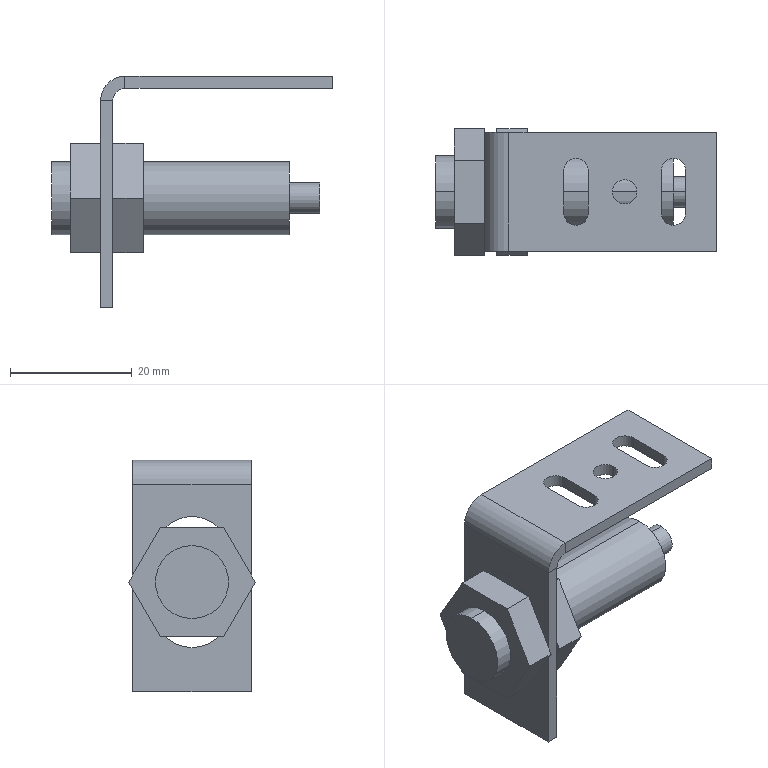Part | STEP file | M12 laser diffuse reflection sensor 1001 | 4 solids | 56 faces | box 46 x 20.785 x 38 mm | volume 8362 mm3 | plane 37 | cylinder 19 | commonest cylinder face diameters 4 x7 12 x6 12.5 x3 5 x2 8 x1